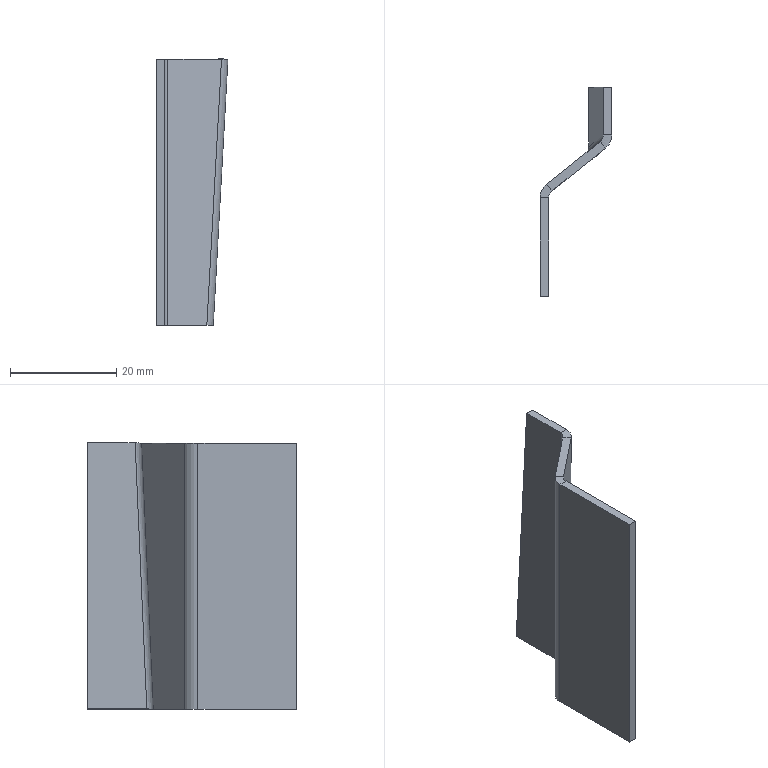Part | SolidWorks | features Fillet 2, Blend 1, FlatPattern 1, SheetMetal 1, SolidToSheetMetal 1 | 1 solid | 22 faces | box 13.5 x 39.3 x 50.088 mm | volume 3525 mm3 | plane 16 | cylinder 4 | spline 2 | commonest cylinder face diameters 3.2 x2 6.4 x2
STEP:
#1=CARTESIAN_POINT('',(-0.3965,21.031,50.));
#2=VERTEX_POINT('',#1);
#3=CARTESIAN_POINT('',(0.6018,19.78,50.));
#4=VERTEX_POINT('',#3);
#5=CARTESIAN_POINT('',(-0.3965,21.031,50.));
#6=CARTESIAN_POINT('',(-0.06372,20.614,50.));
#7=CARTESIAN_POINT('',(0.269,20.197,50.));
#8=CARTESIAN_POINT('',(0.6018,19.78,50.));
#9=B_SPLINE_CURVE_WITH_KNOTS('',3,(#5,#6,#7,#8),.UNSPECIFIED.,.F.,.F.,(4,4),(0.,1.),.UNSPECIFIED.);
#10=EDGE_CURVE('',#2,#4,#9,.T.);
#11=ORIENTED_EDGE('',*,*,#10,.F.);
#12=CARTESIAN_POINT('',(-1.6,18.53,50.));
#13=VERTEX_POINT('',#12);
#14=CARTESIAN_POINT('',(1.6,18.53,50.));
#15=DIRECTION('',(0.,0.,-1.));
#16=DIRECTION('',(0.,-1.,0.));
#17=AXIS2_PLACEMENT_3D('',#14,#15,#16);
#18=CIRCLE('',#17,3.2);
#19=EDGE_CURVE('',#13,#2,#18,.T.);
#20=ORIENTED_EDGE('',*,*,#19,.F.);
#21=CARTESIAN_POINT('',(0.,18.53,50.));
#22=VERTEX_POINT('',#21);
#23=CARTESIAN_POINT('',(-1.6,18.53,50.));
#24=CARTESIAN_POINT('',(-1.067,18.53,50.));
#25=CARTESIAN_POINT('',(-0.5333,18.53,50.));
#26=CARTESIAN_POINT('',(0.,18.53,50.));
#27=B_SPLINE_CURVE_WITH_KNOTS('',3,(#23,#24,#25,#26),.UNSPECIFIED.,.F.,.F.,(4,4),(0.,1.),.UNSPECIFIED.);
#28=EDGE_CURVE('',#13,#22,#27,.T.);
#29=ORIENTED_EDGE('',*,*,#28,.T.);
#30=CARTESIAN_POINT('',(1.6,18.53,50.));
#31=DIRECTION('',(0.,0.,-1.));
#32=DIRECTION('',(-1.,0.,0.));
#33=AXIS2_PLACEMENT_3D('',#30,#31,#32);
#34=CIRCLE('',#33,1.6);
#35=EDGE_CURVE('',#22,#4,#34,.T.);
#36=ORIENTED_EDGE('',*,*,#35,.T.);
#37=EDGE_LOOP('',(#11,#20,#29,#36));
#38=FACE_OUTER_BOUND('',#37,.T.);
#39=CARTESIAN_POINT('',(1.6,18.53,50.));
#40=DIRECTION('',(0.,0.,1.));
#41=DIRECTION('',(1.,0.,0.));
#42=AXIS2_PLACEMENT_3D('',#39,#40,#41);
#43=PLANE('',#42);
#44=ADVANCED_FACE('',(#38),#43,.T.);
#45=ORIENTED_EDGE('',*,*,#28,.F.);
#46=CARTESIAN_POINT('',(-1.6,0.,50.));
#47=VERTEX_POINT('',#46);
#48=CARTESIAN_POINT('',(-1.6,0.,50.));
#49=CARTESIAN_POINT('',(-1.6,6.177,50.));
#50=CARTESIAN_POINT('',(-1.6,12.353,50.));
#51=CARTESIAN_POINT('',(-1.6,18.53,50.));
#52=B_SPLINE_CURVE_WITH_KNOTS('',3,(#48,#49,#50,#51),.UNSPECIFIED.,.F.,.F.,(4,4),(0.03989,1.),.UNSPECIFIED.);
#53=EDGE_CURVE('',#47,#13,#52,.T.);
#54=ORIENTED_EDGE('',*,*,#53,.F.);
#55=CARTESIAN_POINT('',(0.,0.,50.));
#56=VERTEX_POINT('',#55);
#57=CARTESIAN_POINT('',(-1.6,0.,50.));
#58=CARTESIAN_POINT('',(-1.067,0.,50.));
#59=CARTESIAN_POINT('',(-0.5333,0.,50.));
#60=CARTESIAN_POINT('',(0.,0.,50.));
#61=B_SPLINE_CURVE_WITH_KNOTS('',3,(#57,#58,#59,#60),.UNSPECIFIED.,.F.,.F.,(4,4),(0.,1.),.UNSPECIFIED.);
#62=EDGE_CURVE('',#47,#56,#61,.T.);
#63=ORIENTED_EDGE('',*,*,#62,.T.);
#64=CARTESIAN_POINT('',(0.,0.,50.));
#65=DIRECTION('',(0.,1.,0.));
#66=VECTOR('',#65,1000.);
#67=LINE('',#64,#66);
#68=EDGE_CURVE('',#56,#22,#67,.T.);
#69=ORIENTED_EDGE('',*,*,#68,.T.);
#70=EDGE_LOOP('',(#45,#54,#63,#69));
#71=FACE_OUTER_BOUND('',#70,.T.);
#72=CARTESIAN_POINT('',(0.,18.53,50.));
#73=DIRECTION('',(0.,0.,1.));
#74=DIRECTION('',(-1.,0.,0.));
#75=AXIS2_PLACEMENT_3D('',#72,#73,#74);
#76=PLANE('',#75);
#77=ADVANCED_FACE('',(#71),#76,.T.);
#78=ORIENTED_EDGE('',*,*,#62,.F.);
#79=CARTESIAN_POINT('',(-1.6,0.,0.));
#80=VERTEX_POINT('',#79);
#81=CARTESIAN_POINT('',(-1.6,0.,0.));
#82=DIRECTION('',(0.,0.,-1.));
#83=VECTOR('',#82,1000.);
#84=LINE('',#81,#83);
#85=EDGE_CURVE('',#47,#80,#84,.T.);
#86=ORIENTED_EDGE('',*,*,#85,.T.);
#87=CARTESIAN_POINT('',(0.,0.,0.));
#88=VERTEX_POINT('',#87);
#89=CARTESIAN_POINT('',(-1.6,0.,0.));
#90=CARTESIAN_POINT('',(-1.067,0.,0.));
#91=CARTESIAN_POINT('',(-0.5333,0.,0.));
#92=CARTESIAN_POINT('',(0.,0.,0.));
#93=B_SPLINE_CURVE_WITH_KNOTS('',3,(#89,#90,#91,#92),.UNSPECIFIED.,.F.,.F.,(4,4),(0.,1.),.UNSPECIFIED.);
#94=EDGE_CURVE('',#80,#88,#93,.T.);
#95=ORIENTED_EDGE('',*,*,#94,.T.);
#96=CARTESIAN_POINT('',(0.,0.,50.));
#97=DIRECTION('',(0.,0.,-1.));
#98=VECTOR('',#97,1000.);
#99=LINE('',#96,#98);
#100=EDGE_CURVE('',#56,#88,#99,.T.);
#101=ORIENTED_EDGE('',*,*,#100,.F.);
#102=EDGE_LOOP('',(#78,#86,#95,#101));
#103=FACE_OUTER_BOUND('',#102,.T.);
#104=CARTESIAN_POINT('',(0.,0.,50.));
#105=DIRECTION('',(0.,-1.,0.));
#106=DIRECTION('',(0.,0.,-1.));
#107=AXIS2_PLACEMENT_3D('',#104,#105,#106);
#108=PLANE('',#107);
#109=ADVANCED_FACE('',(#103),#108,.T.);
#110=ORIENTED_EDGE('',*,*,#94,.F.);
#111=CARTESIAN_POINT('',(-1.6,18.53,0.));
#112=VERTEX_POINT('',#111);
#113=CARTESIAN_POINT('',(-1.6,0.,0.));
#114=CARTESIAN_POINT('',(-1.6,6.177,0.));
#115=CARTESIAN_POINT('',(-1.6,12.353,0.));
#116=CARTESIAN_POINT('',(-1.6,18.53,0.));
#117=B_SPLINE_CURVE_WITH_KNOTS('',3,(#113,#114,#115,#116),.UNSPECIFIED.,.F.,.F.,(4,4),(0.,1.),.UNSPECIFIED.);
#118=EDGE_CURVE('',#80,#112,#117,.T.);
#119=ORIENTED_EDGE('',*,*,#118,.T.);
#120=CARTESIAN_POINT('',(0.,18.53,0.));
#121=VERTEX_POINT('',#120);
#122=CARTESIAN_POINT('',(-1.6,18.53,0.));
#123=CARTESIAN_POINT('',(-1.067,18.53,0.));
#124=CARTESIAN_POINT('',(-0.5333,18.53,0.));
#125=CARTESIAN_POINT('',(0.,18.53,0.));
#126=B_SPLINE_CURVE_WITH_KNOTS('',3,(#122,#123,#124,#125),.UNSPECIFIED.,.F.,.F.,(4,4),(0.,1.),.UNSPECIFIED.);
#127=EDGE_CURVE('',#112,#121,#126,.T.);
#128=ORIENTED_EDGE('',*,*,#127,.T.);
#129=CARTESIAN_POINT('',(0.,19.3,0.));
#130=DIRECTION('',(0.,1.,0.));
#131=VECTOR('',#130,1000.);
#132=LINE('',#129,#131);
#133=EDGE_CURVE('',#88,#121,#132,.T.);
#134=ORIENTED_EDGE('',*,*,#133,.F.);
#135=EDGE_LOOP('',(#110,#119,#128,#134));
#136=FACE_OUTER_BOUND('',#135,.T.);
#137=CARTESIAN_POINT('',(0.,0.,0.));
#138=DIRECTION('',(0.,0.,-1.));
#139=DIRECTION('',(-1.,0.,0.));
#140=AXIS2_PLACEMENT_3D('',#137,#138,#139);
#141=PLANE('',#140);
#142=ADVANCED_FACE('',(#136),#141,.T.);
#143=ORIENTED_EDGE('',*,*,#127,.F.);
#144=CARTESIAN_POINT('',(-0.3965,21.031,0.));
#145=VERTEX_POINT('',#144);
#146=CARTESIAN_POINT('',(1.6,18.53,0.));
#147=DIRECTION('',(0.,0.,1.));
#148=DIRECTION('',(0.,-1.,0.));
#149=AXIS2_PLACEMENT_3D('',#146,#147,#148);
#150=CIRCLE('',#149,3.2);
#151=EDGE_CURVE('',#145,#112,#150,.T.);
#152=ORIENTED_EDGE('',*,*,#151,.F.);
#153=CARTESIAN_POINT('',(0.6018,19.78,0.));
#154=VERTEX_POINT('',#153);
#155=CARTESIAN_POINT('',(-0.3965,21.031,0.));
#156=CARTESIAN_POINT('',(-0.06372,20.614,0.));
#157=CARTESIAN_POINT('',(0.269,20.197,0.));
#158=CARTESIAN_POINT('',(0.6018,19.78,0.));
#159=B_SPLINE_CURVE_WITH_KNOTS('',3,(#155,#156,#157,#158),.UNSPECIFIED.,.F.,.F.,(4,4),(0.,1.),.UNSPECIFIED.);
#160=EDGE_CURVE('',#145,#154,#159,.T.);
#161=ORIENTED_EDGE('',*,*,#160,.T.);
#162=CARTESIAN_POINT('',(1.6,18.53,0.));
#163=DIRECTION('',(0.,0.,1.));
#164=DIRECTION('',(1.,0.,0.));
#165=AXIS2_PLACEMENT_3D('',#162,#163,#164);
#166=CIRCLE('',#165,1.6);
#167=EDGE_CURVE('',#154,#121,#166,.T.);
#168=ORIENTED_EDGE('',*,*,#167,.T.);
#169=EDGE_LOOP('',(#143,#152,#161,#168));
#170=FACE_OUTER_BOUND('',#169,.T.);
#171=CARTESIAN_POINT('',(1.6,18.53,0.));
#172=DIRECTION('',(0.,0.,-1.));
#173=DIRECTION('',(-1.,0.,0.));
#174=AXIS2_PLACEMENT_3D('',#171,#172,#173);
#175=PLANE('',#174);
#176=ADVANCED_FACE('',(#170),#175,.T.);
#177=ORIENTED_EDGE('',*,*,#160,.F.);
#178=CARTESIAN_POINT('',(6.938,26.886,0.));
#179=VERTEX_POINT('',#178);
#180=CARTESIAN_POINT('',(-0.3965,21.031,0.));
#181=CARTESIAN_POINT('',(2.048,22.982,0.));
#182=CARTESIAN_POINT('',(4.493,24.934,0.));
#183=CARTESIAN_POINT('',(6.938,26.886,0.));
#184=B_SPLINE_CURVE_WITH_KNOTS('',3,(#180,#181,#182,#183),.UNSPECIFIED.,.F.,.F.,(4,4),(0.,1.),.UNSPECIFIED.);
#185=EDGE_CURVE('',#145,#179,#184,.T.);
#186=ORIENTED_EDGE('',*,*,#185,.T.);
#187=CARTESIAN_POINT('',(7.936,25.635,0.));
#188=VERTEX_POINT('',#187);
#189=CARTESIAN_POINT('',(6.938,26.886,0.));
#190=CARTESIAN_POINT('',(7.27,26.469,0.));
#191=CARTESIAN_POINT('',(7.603,26.052,0.));
#192=CARTESIAN_POINT('',(7.936,25.635,0.));
#193=B_SPLINE_CURVE_WITH_KNOTS('',3,(#189,#190,#191,#192),.UNSPECIFIED.,.F.,.F.,(4,4),(0.,1.),.UNSPECIFIED.);
#194=EDGE_CURVE('',#179,#188,#193,.T.);
#195=ORIENTED_EDGE('',*,*,#194,.T.);
#196=CARTESIAN_POINT('',(0.,19.3,0.));
#197=DIRECTION('',(0.7815,0.6239,0.));
#198=VECTOR('',#197,1000.);
#199=LINE('',#196,#198);
#200=EDGE_CURVE('',#154,#188,#199,.T.);
#201=ORIENTED_EDGE('',*,*,#200,.F.);
#202=EDGE_LOOP('',(#177,#186,#195,#201));
#203=FACE_OUTER_BOUND('',#202,.T.);
#204=CARTESIAN_POINT('',(0.6018,19.78,0.));
#205=DIRECTION('',(0.,0.,-1.));
#206=DIRECTION('',(-0.6239,0.7815,0.));
#207=AXIS2_PLACEMENT_3D('',#204,#205,#206);
#208=PLANE('',#207);
#209=ADVANCED_FACE('',(#203),#208,.T.);
#210=ORIENTED_EDGE('',*,*,#194,.F.);
#211=CARTESIAN_POINT('',(7.547,28.144,0.08805));
#212=VERTEX_POINT('',#211);
#213=CARTESIAN_POINT('',(7.547,28.144,0.08805));
#214=CARTESIAN_POINT('',(7.545,27.647,0.06632));
#215=CARTESIAN_POINT('',(7.328,27.197,0.03489));
#216=CARTESIAN_POINT('',(6.938,26.886,0.));
#217=(BOUNDED_CURVE()B_SPLINE_CURVE(3,(#213,#214,#215,#216),.UNSPECIFIED.,.F.,.F.)B_SPLINE_CURVE_WITH_KNOTS((4,4),(3.814,4.712),.UNSPECIFIED.)CURVE()GEOMETRIC_REPRESENTATION_ITEM()RATIONAL_B_SPLINE_CURVE((1.,0.9339,0.9339,1.))REPRESENTATION_ITEM(''));
#218=EDGE_CURVE('',#212,#179,#217,.T.);
#219=ORIENTED_EDGE('',*,*,#218,.F.);
#220=CARTESIAN_POINT('',(9.144,28.144,0.));
#221=VERTEX_POINT('',#220);
#222=CARTESIAN_POINT('',(7.547,28.144,0.08805));
#223=CARTESIAN_POINT('',(8.079,28.144,0.0587));
#224=CARTESIAN_POINT('',(8.612,28.144,0.02935));
#225=CARTESIAN_POINT('',(9.144,28.144,0.));
#226=(BOUNDED_CURVE()B_SPLINE_CURVE(3,(#222,#223,#224,#225),.UNSPECIFIED.,.F.,.F.)B_SPLINE_CURVE_WITH_KNOTS((4,4),(0.,1.),.UNSPECIFIED.)CURVE()GEOMETRIC_REPRESENTATION_ITEM()RATIONAL_B_SPLINE_CURVE((0.6162,0.6162,0.6162,0.6162))REPRESENTATION_ITEM(''));
#227=EDGE_CURVE('',#212,#221,#226,.T.);
#228=ORIENTED_EDGE('',*,*,#227,.T.);
#229=CARTESIAN_POINT('',(9.144,28.144,0.));
#230=CARTESIAN_POINT('',(9.144,27.151,0.));
#231=CARTESIAN_POINT('',(8.713,26.256,0.));
#232=CARTESIAN_POINT('',(7.936,25.635,0.));
#233=(BOUNDED_CURVE()B_SPLINE_CURVE(3,(#229,#230,#231,#232),.UNSPECIFIED.,.F.,.F.)B_SPLINE_CURVE_WITH_KNOTS((4,4),(3.814,4.712),.UNSPECIFIED.)CURVE()GEOMETRIC_REPRESENTATION_ITEM()RATIONAL_B_SPLINE_CURVE((1.,0.9339,0.9339,1.))REPRESENTATION_ITEM(''));
#234=EDGE_CURVE('',#221,#188,#233,.T.);
#235=ORIENTED_EDGE('',*,*,#234,.T.);
#236=EDGE_LOOP('',(#210,#219,#228,#235));
#237=FACE_OUTER_BOUND('',#236,.T.);
#238=CARTESIAN_POINT('',(3.432,26.135,0.));
#239=CARTESIAN_POINT('',(3.848,26.467,-0.03752));
#240=CARTESIAN_POINT('',(4.264,26.799,-0.07504));
#241=CARTESIAN_POINT('',(4.68,27.13,-0.1126));
#242=CARTESIAN_POINT('',(-0.5606,31.136,0.));
#243=CARTESIAN_POINT('',(0.5207,30.635,-0.03752));
#244=CARTESIAN_POINT('',(1.602,30.133,-0.07504));
#245=CARTESIAN_POINT('',(2.683,29.631,-0.1126));
#246=CARTESIAN_POINT('',(4.453,35.139,0.));
#247=CARTESIAN_POINT('',(4.703,33.974,0.03752));
#248=CARTESIAN_POINT('',(4.953,32.808,0.07504));
#249=CARTESIAN_POINT('',(5.203,31.643,0.1126));
#250=CARTESIAN_POINT('',(8.446,30.138,0.));
#251=CARTESIAN_POINT('',(8.031,29.806,0.03752));
#252=CARTESIAN_POINT('',(7.615,29.474,0.07504));
#253=CARTESIAN_POINT('',(7.199,29.142,0.1126));
#254=CARTESIAN_POINT('',(12.439,25.136,0.));
#255=CARTESIAN_POINT('',(11.358,25.638,0.03752));
#256=CARTESIAN_POINT('',(10.277,26.139,0.07504));
#257=CARTESIAN_POINT('',(9.196,26.641,0.1126));
#258=CARTESIAN_POINT('',(7.425,21.133,0.));
#259=CARTESIAN_POINT('',(7.176,22.299,-0.03752));
#260=CARTESIAN_POINT('',(6.926,23.464,-0.07504));
#261=CARTESIAN_POINT('',(6.676,24.63,-0.1126));
#262=CARTESIAN_POINT('',(3.432,26.135,0.));
#263=CARTESIAN_POINT('',(3.848,26.467,-0.03752));
#264=CARTESIAN_POINT('',(4.264,26.799,-0.07504));
#265=CARTESIAN_POINT('',(4.68,27.13,-0.1126));
#266=(BOUNDED_SURFACE()B_SPLINE_SURFACE(3,3,((#238,#239,#240,#241),(#242,#243,#244,#245),(#246,#247,#248,#249),(#250,#251,#252,#253),(#254,#255,#256,#257),(#258,#259,#260,#261),(#262,#263,#264,#265)),.UNSPECIFIED.,.T.,.F.,.F.)B_SPLINE_SURFACE_WITH_KNOTS((4,3,4),(4,4),(0.,0.5,1.),(0.,1.),.UNSPECIFIED.)GEOMETRIC_REPRESENTATION_ITEM()RATIONAL_B_SPLINE_SURFACE(((1.,1.,1.,1.),(0.3333,0.3333,0.3333,0.3333),(0.3333,0.3333,0.3333,0.3333),(1.,1.,1.,1.),(0.3333,0.3333,0.3333,0.3333),(0.3333,0.3333,0.3333,0.3333),(1.,1.,1.,1.)))REPRESENTATION_ITEM('')SURFACE());
#267=ADVANCED_FACE('',(#237),#266,.T.);
#268=ORIENTED_EDGE('',*,*,#227,.F.);
#269=CARTESIAN_POINT('',(7.547,39.3,0.08805));
#270=VERTEX_POINT('',#269);
#271=CARTESIAN_POINT('',(7.547,28.144,0.08805));
#272=CARTESIAN_POINT('',(7.547,31.863,0.08805));
#273=CARTESIAN_POINT('',(7.547,35.581,0.08805));
#274=CARTESIAN_POINT('',(7.547,39.3,0.08805));
#275=B_SPLINE_CURVE_WITH_KNOTS('',3,(#271,#272,#273,#274),.UNSPECIFIED.,.F.,.F.,(4,4),(0.,1.),.UNSPECIFIED.);
#276=EDGE_CURVE('',#212,#270,#275,.T.);
#277=ORIENTED_EDGE('',*,*,#276,.T.);
#278=CARTESIAN_POINT('',(9.144,39.3,0.));
#279=VERTEX_POINT('',#278);
#280=CARTESIAN_POINT('',(7.547,39.3,0.08805));
#281=CARTESIAN_POINT('',(8.079,39.3,0.0587));
#282=CARTESIAN_POINT('',(8.612,39.3,0.02935));
#283=CARTESIAN_POINT('',(9.144,39.3,0.));
#284=B_SPLINE_CURVE_WITH_KNOTS('',3,(#280,#281,#282,#283),.UNSPECIFIED.,.F.,.F.,(4,4),(0.,1.),.UNSPECIFIED.);
#285=EDGE_CURVE('',#270,#279,#284,.T.);
#286=ORIENTED_EDGE('',*,*,#285,.T.);
#287=CARTESIAN_POINT('',(9.144,39.3,0.));
#288=DIRECTION('',(0.,1.,0.));
#289=VECTOR('',#288,1000.);
#290=LINE('',#287,#289);
#291=EDGE_CURVE('',#221,#279,#290,.T.);
#292=ORIENTED_EDGE('',*,*,#291,.F.);
#293=EDGE_LOOP('',(#268,#277,#286,#292));
#294=FACE_OUTER_BOUND('',#293,.T.);
#295=CARTESIAN_POINT('',(9.144,28.144,0.));
#296=DIRECTION('',(-0.05503,0.,-0.9985));
#297=DIRECTION('',(-0.9985,0.,0.05503));
#298=AXIS2_PLACEMENT_3D('',#295,#296,#297);
#299=PLANE('',#298);
#300=ADVANCED_FACE('',(#294),#299,.T.);
#301=ORIENTED_EDGE('',*,*,#285,.F.);
#302=CARTESIAN_POINT('',(10.302,39.3,50.088));
#303=VERTEX_POINT('',#302);
#304=CARTESIAN_POINT('',(7.519,39.3,-0.4144));
#305=DIRECTION('',(-0.05503,0.,-0.9985));
#306=VECTOR('',#305,1000.);
#307=LINE('',#304,#306);
#308=EDGE_CURVE('',#303,#270,#307,.T.);
#309=ORIENTED_EDGE('',*,*,#308,.F.);
#310=CARTESIAN_POINT('',(11.9,39.3,50.));
#311=VERTEX_POINT('',#310);
#312=CARTESIAN_POINT('',(10.302,39.3,50.088));
#313=CARTESIAN_POINT('',(10.835,39.3,50.059));
#314=CARTESIAN_POINT('',(11.367,39.3,50.029));
#315=CARTESIAN_POINT('',(11.9,39.3,50.));
#316=B_SPLINE_CURVE_WITH_KNOTS('',3,(#312,#313,#314,#315),.UNSPECIFIED.,.F.,.F.,(4,4),(0.,1.),.UNSPECIFIED.);
#317=EDGE_CURVE('',#303,#311,#316,.T.);
#318=ORIENTED_EDGE('',*,*,#317,.T.);
#319=CARTESIAN_POINT('',(11.9,39.3,50.));
#320=DIRECTION('',(-0.05503,0.,-0.9985));
#321=VECTOR('',#320,1000.);
#322=LINE('',#319,#321);
#323=EDGE_CURVE('',#311,#279,#322,.T.);
#324=ORIENTED_EDGE('',*,*,#323,.T.);
#325=EDGE_LOOP('',(#301,#309,#318,#324));
#326=FACE_OUTER_BOUND('',#325,.T.);
#327=CARTESIAN_POINT('',(11.9,39.3,50.));
#328=DIRECTION('',(0.,-1.,0.));
#329=DIRECTION('',(-0.05503,0.,-0.9985));
#330=AXIS2_PLACEMENT_3D('',#327,#328,#329);
#331=PLANE('',#330);
#332=ADVANCED_FACE('',(#326),#331,.F.);
#333=ORIENTED_EDGE('',*,*,#317,.F.);
#334=CARTESIAN_POINT('',(10.302,30.344,50.088));
#335=VERTEX_POINT('',#334);
#336=CARTESIAN_POINT('',(10.302,30.344,50.088));
#337=CARTESIAN_POINT('',(10.302,33.329,50.088));
#338=CARTESIAN_POINT('',(10.302,36.315,50.088));
#339=CARTESIAN_POINT('',(10.302,39.3,50.088));
#340=B_SPLINE_CURVE_WITH_KNOTS('',3,(#336,#337,#338,#339),.UNSPECIFIED.,.F.,.F.,(4,4),(0.0000024,0.853),.UNSPECIFIED.);
#341=EDGE_CURVE('',#335,#303,#340,.T.);
#342=ORIENTED_EDGE('',*,*,#341,.F.);
#343=CARTESIAN_POINT('',(11.9,30.344,50.));
#344=VERTEX_POINT('',#343);
#345=CARTESIAN_POINT('',(10.302,30.344,50.088));
#346=CARTESIAN_POINT('',(10.835,30.344,50.059));
#347=CARTESIAN_POINT('',(11.367,30.344,50.029));
#348=CARTESIAN_POINT('',(11.9,30.344,50.));
#349=B_SPLINE_CURVE_WITH_KNOTS('',3,(#345,#346,#347,#348),.UNSPECIFIED.,.F.,.F.,(4,4),(0.,1.),.UNSPECIFIED.);
#350=EDGE_CURVE('',#335,#344,#349,.T.);
#351=ORIENTED_EDGE('',*,*,#350,.T.);
#352=CARTESIAN_POINT('',(11.9,39.3,50.));
#353=DIRECTION('',(0.,1.,0.));
#354=VECTOR('',#353,1000.);
#355=LINE('',#352,#354);
#356=EDGE_CURVE('',#344,#311,#355,.T.);
#357=ORIENTED_EDGE('',*,*,#356,.T.);
#358=EDGE_LOOP('',(#333,#342,#351,#357));
#359=FACE_OUTER_BOUND('',#358,.T.);
#360=CARTESIAN_POINT('',(11.9,39.3,50.));
#361=DIRECTION('',(0.05503,0.,0.9985));
#362=DIRECTION('',(-0.9985,0.,0.05503));
#363=AXIS2_PLACEMENT_3D('',#360,#361,#362);
#364=PLANE('',#363);
#365=ADVANCED_FACE('',(#359),#364,.T.);
#366=ORIENTED_EDGE('',*,*,#350,.F.);
#367=CARTESIAN_POINT('',(9.693,29.086,50.));
#368=VERTEX_POINT('',#367);
#369=CARTESIAN_POINT('',(9.693,29.086,50.));
#370=CARTESIAN_POINT('',(10.084,29.397,50.035));
#371=CARTESIAN_POINT('',(10.301,29.847,50.066));
#372=CARTESIAN_POINT('',(10.302,30.344,50.088));
#373=(BOUNDED_CURVE()B_SPLINE_CURVE(3,(#369,#370,#371,#372),.UNSPECIFIED.,.F.,.F.)B_SPLINE_CURVE_WITH_KNOTS((4,4),(1.571,2.469),.UNSPECIFIED.)CURVE()GEOMETRIC_REPRESENTATION_ITEM()RATIONAL_B_SPLINE_CURVE((1.,0.9339,0.9339,1.))REPRESENTATION_ITEM(''));
#374=EDGE_CURVE('',#368,#335,#373,.T.);
#375=ORIENTED_EDGE('',*,*,#374,.F.);
#376=CARTESIAN_POINT('',(10.692,27.835,50.));
#377=VERTEX_POINT('',#376);
#378=CARTESIAN_POINT('',(9.693,29.086,50.));
#379=CARTESIAN_POINT('',(10.026,28.669,50.));
#380=CARTESIAN_POINT('',(10.359,28.252,50.));
#381=CARTESIAN_POINT('',(10.692,27.835,50.));
#382=(BOUNDED_CURVE()B_SPLINE_CURVE(3,(#378,#379,#380,#381),.UNSPECIFIED.,.F.,.F.)B_SPLINE_CURVE_WITH_KNOTS((4,4),(0.,1.),.UNSPECIFIED.)CURVE()GEOMETRIC_REPRESENTATION_ITEM()RATIONAL_B_SPLINE_CURVE((0.5,0.5,0.5,0.5))REPRESENTATION_ITEM(''));
#383=EDGE_CURVE('',#368,#377,#382,.T.);
#384=ORIENTED_EDGE('',*,*,#383,.T.);
#385=CARTESIAN_POINT('',(10.692,27.835,50.));
#386=CARTESIAN_POINT('',(11.469,28.456,50.));
#387=CARTESIAN_POINT('',(11.9,29.351,50.));
#388=CARTESIAN_POINT('',(11.9,30.344,50.));
#389=(BOUNDED_CURVE()B_SPLINE_CURVE(3,(#385,#386,#387,#388),.UNSPECIFIED.,.F.,.F.)B_SPLINE_CURVE_WITH_KNOTS((4,4),(1.571,2.469),.UNSPECIFIED.)CURVE()GEOMETRIC_REPRESENTATION_ITEM()RATIONAL_B_SPLINE_CURVE((1.,0.9339,0.9339,1.))REPRESENTATION_ITEM(''));
#390=EDGE_CURVE('',#377,#344,#389,.T.);
#391=ORIENTED_EDGE('',*,*,#390,.T.);
#392=EDGE_LOOP('',(#366,#375,#384,#391));
#393=FACE_OUTER_BOUND('',#392,.T.);
#394=CARTESIAN_POINT('',(6.188,28.335,50.));
#395=CARTESIAN_POINT('',(6.604,28.667,49.962));
#396=CARTESIAN_POINT('',(7.02,28.999,49.925));
#397=CARTESIAN_POINT('',(7.435,29.33,49.887));
#398=CARTESIAN_POINT('',(10.181,23.333,50.));
#399=CARTESIAN_POINT('',(9.931,24.499,49.962));
#400=CARTESIAN_POINT('',(9.682,25.664,49.925));
#401=CARTESIAN_POINT('',(9.432,26.83,49.887));
#402=CARTESIAN_POINT('',(15.195,27.336,50.));
#403=CARTESIAN_POINT('',(14.114,27.838,50.038));
#404=CARTESIAN_POINT('',(13.033,28.339,50.075));
#405=CARTESIAN_POINT('',(11.951,28.841,50.113));
#406=CARTESIAN_POINT('',(11.202,32.338,50.));
#407=CARTESIAN_POINT('',(10.786,32.006,50.038));
#408=CARTESIAN_POINT('',(10.371,31.674,50.075));
#409=CARTESIAN_POINT('',(9.955,31.342,50.113));
#410=CARTESIAN_POINT('',(7.209,37.339,50.));
#411=CARTESIAN_POINT('',(7.459,36.174,50.038));
#412=CARTESIAN_POINT('',(7.709,35.008,50.075));
#413=CARTESIAN_POINT('',(7.958,33.843,50.113));
#414=CARTESIAN_POINT('',(2.195,33.336,50.));
#415=CARTESIAN_POINT('',(3.276,32.835,49.962));
#416=CARTESIAN_POINT('',(4.358,32.333,49.925));
#417=CARTESIAN_POINT('',(5.439,31.831,49.887));
#418=CARTESIAN_POINT('',(6.188,28.335,50.));
#419=CARTESIAN_POINT('',(6.604,28.667,49.962));
#420=CARTESIAN_POINT('',(7.02,28.999,49.925));
#421=CARTESIAN_POINT('',(7.435,29.33,49.887));
#422=(BOUNDED_SURFACE()B_SPLINE_SURFACE(3,3,((#394,#395,#396,#397),(#398,#399,#400,#401),(#402,#403,#404,#405),(#406,#407,#408,#409),(#410,#411,#412,#413),(#414,#415,#416,#417),(#418,#419,#420,#421)),.UNSPECIFIED.,.T.,.F.,.F.)B_SPLINE_SURFACE_WITH_KNOTS((4,3,4),(4,4),(0.,0.5,1.),(0.,1.),.UNSPECIFIED.)GEOMETRIC_REPRESENTATION_ITEM()RATIONAL_B_SPLINE_SURFACE(((1.,1.,1.,1.),(0.3333,0.3333,0.3333,0.3333),(0.3333,0.3333,0.3333,0.3333),(1.,1.,1.,1.),(0.3333,0.3333,0.3333,0.3333),(0.3333,0.3333,0.3333,0.3333),(1.,1.,1.,1.)))REPRESENTATION_ITEM('')SURFACE());
#423=ADVANCED_FACE('',(#393),#422,.T.);
#424=CARTESIAN_POINT('',(-0.3965,21.031,50.));
#425=CARTESIAN_POINT('',(2.967,23.716,50.));
#426=CARTESIAN_POINT('',(6.33,26.401,50.));
#427=CARTESIAN_POINT('',(9.693,29.086,50.));
#428=B_SPLINE_CURVE_WITH_KNOTS('',3,(#424,#425,#426,#427),.UNSPECIFIED.,.F.,.F.,(4,4),(0.1015,0.9494),.UNSPECIFIED.);
#429=EDGE_CURVE('',#2,#368,#428,.T.);
#430=ORIENTED_EDGE('',*,*,#429,.F.);
#431=ORIENTED_EDGE('',*,*,#10,.T.);
#432=CARTESIAN_POINT('',(0.,19.3,50.));
#433=DIRECTION('',(0.7815,0.6239,0.));
#434=VECTOR('',#433,1000.);
#435=LINE('',#432,#434);
#436=EDGE_CURVE('',#4,#377,#435,.T.);
#437=ORIENTED_EDGE('',*,*,#436,.T.);
#438=ORIENTED_EDGE('',*,*,#383,.F.);
#439=EDGE_LOOP('',(#430,#431,#437,#438));
#440=FACE_OUTER_BOUND('',#439,.T.);
#441=CARTESIAN_POINT('',(10.692,27.835,50.));
#442=DIRECTION('',(0.,0.,1.));
#443=DIRECTION('',(-0.6239,0.7815,0.));
#444=AXIS2_PLACEMENT_3D('',#441,#442,#443);
#445=PLANE('',#444);
#446=ADVANCED_FACE('',(#440),#445,.T.);
#447=ORIENTED_EDGE('',*,*,#390,.F.);
#448=CARTESIAN_POINT('',(7.85,25.567,-1.558));
#449=DIRECTION('',(0.05498,0.04389,0.9975));
#450=VECTOR('',#449,1000.);
#451=LINE('',#448,#450);
#452=EDGE_CURVE('',#188,#377,#451,.T.);
#453=ORIENTED_EDGE('',*,*,#452,.F.);
#454=ORIENTED_EDGE('',*,*,#234,.F.);
#455=CARTESIAN_POINT('',(9.049,28.068,-1.734));
#456=DIRECTION('',(-0.05498,-0.04389,-0.9975));
#457=VECTOR('',#456,1000.);
#458=LINE('',#455,#457);
#459=EDGE_CURVE('',#344,#221,#458,.T.);
#460=ORIENTED_EDGE('',*,*,#459,.F.);
#461=EDGE_LOOP('',(#447,#453,#454,#460));
#462=FACE_OUTER_BOUND('',#461,.T.);
#463=CARTESIAN_POINT('',(5.854,28.068,-1.558));
#464=DIRECTION('',(-0.05498,-0.04389,-0.9975));
#465=DIRECTION('',(-0.9985,0.,0.05503));
#466=AXIS2_PLACEMENT_3D('',#463,#464,#465);
#467=CYLINDRICAL_SURFACE('',#466,3.2);
#468=ADVANCED_FACE('',(#462),#467,.T.);
#469=ORIENTED_EDGE('',*,*,#356,.F.);
#470=ORIENTED_EDGE('',*,*,#459,.T.);
#471=ORIENTED_EDGE('',*,*,#291,.T.);
#472=ORIENTED_EDGE('',*,*,#323,.F.);
#473=EDGE_LOOP('',(#469,#470,#471,#472));
#474=FACE_OUTER_BOUND('',#473,.T.);
#475=CARTESIAN_POINT('',(9.117,0.,-0.5025));
#476=DIRECTION('',(0.9985,0.,-0.05503));
#477=DIRECTION('',(-0.05503,0.,-0.9985));
#478=AXIS2_PLACEMENT_3D('',#475,#476,#477);
#479=PLANE('',#478);
#480=ADVANCED_FACE('',(#474),#479,.T.);
#481=ORIENTED_EDGE('',*,*,#35,.F.);
#482=CARTESIAN_POINT('',(0.,18.53,50.));
#483=DIRECTION('',(0.,0.,1.));
#484=VECTOR('',#483,1000.);
#485=LINE('',#482,#484);
#486=EDGE_CURVE('',#121,#22,#485,.T.);
#487=ORIENTED_EDGE('',*,*,#486,.F.);
#488=ORIENTED_EDGE('',*,*,#167,.F.);
#489=CARTESIAN_POINT('',(0.6018,19.78,0.));
#490=DIRECTION('',(0.,0.,-1.));
#491=VECTOR('',#490,1000.);
#492=LINE('',#489,#491);
#493=EDGE_CURVE('',#4,#154,#492,.T.);
#494=ORIENTED_EDGE('',*,*,#493,.F.);
#495=EDGE_LOOP('',(#481,#487,#488,#494));
#496=FACE_OUTER_BOUND('',#495,.T.);
#497=CARTESIAN_POINT('',(1.6,18.53,0.));
#498=DIRECTION('',(0.,0.,1.));
#499=DIRECTION('',(0.,-1.,0.));
#500=AXIS2_PLACEMENT_3D('',#497,#498,#499);
#501=CYLINDRICAL_SURFACE('',#500,1.6);
#502=ADVANCED_FACE('',(#496),#501,.F.);
#503=ORIENTED_EDGE('',*,*,#200,.T.);
#504=ORIENTED_EDGE('',*,*,#452,.T.);
#505=ORIENTED_EDGE('',*,*,#436,.F.);
#506=ORIENTED_EDGE('',*,*,#493,.T.);
#507=EDGE_LOOP('',(#503,#504,#505,#506));
#508=FACE_OUTER_BOUND('',#507,.T.);
#509=CARTESIAN_POINT('',(-9.41,11.788,0.));
#510=DIRECTION('',(0.6239,-0.7815,0.));
#511=DIRECTION('',(0.7815,0.6239,0.));
#512=AXIS2_PLACEMENT_3D('',#509,#510,#511);
#513=PLANE('',#512);
#514=ADVANCED_FACE('',(#508),#513,.T.);
#515=ORIENTED_EDGE('',*,*,#133,.T.);
#516=ORIENTED_EDGE('',*,*,#486,.T.);
#517=ORIENTED_EDGE('',*,*,#68,.F.);
#518=ORIENTED_EDGE('',*,*,#100,.T.);
#519=EDGE_LOOP('',(#515,#516,#517,#518));
#520=FACE_OUTER_BOUND('',#519,.T.);
#521=CARTESIAN_POINT('',(0.,0.,0.));
#522=DIRECTION('',(1.,0.,0.));
#523=DIRECTION('',(0.,1.,0.));
#524=AXIS2_PLACEMENT_3D('',#521,#522,#523);
#525=PLANE('',#524);
#526=ADVANCED_FACE('',(#520),#525,.T.);
#527=ORIENTED_EDGE('',*,*,#374,.T.);
#528=CARTESIAN_POINT('',(7.451,28.068,-1.646));
#529=DIRECTION('',(-0.05498,-0.04389,-0.9975));
#530=VECTOR('',#529,1000.);
#531=LINE('',#528,#530);
#532=EDGE_CURVE('',#335,#212,#531,.T.);
#533=ORIENTED_EDGE('',*,*,#532,.T.);
#534=ORIENTED_EDGE('',*,*,#218,.T.);
#535=CARTESIAN_POINT('',(6.852,26.817,-1.558));
#536=DIRECTION('',(0.05498,0.04389,0.9975));
#537=VECTOR('',#536,1000.);
#538=LINE('',#535,#537);
#539=EDGE_CURVE('',#179,#368,#538,.T.);
#540=ORIENTED_EDGE('',*,*,#539,.T.);
#541=EDGE_LOOP('',(#527,#533,#534,#540));
#542=FACE_OUTER_BOUND('',#541,.T.);
#543=CARTESIAN_POINT('',(5.854,28.068,-1.558));
#544=DIRECTION('',(-0.05498,-0.04389,-0.9975));
#545=DIRECTION('',(-0.9985,0.,0.05503));
#546=AXIS2_PLACEMENT_3D('',#543,#544,#545);
#547=CYLINDRICAL_SURFACE('',#546,1.6);
#548=ADVANCED_FACE('',(#542),#547,.F.);
#549=ORIENTED_EDGE('',*,*,#341,.T.);
#550=ORIENTED_EDGE('',*,*,#308,.T.);
#551=ORIENTED_EDGE('',*,*,#276,.F.);
#552=ORIENTED_EDGE('',*,*,#532,.F.);
#553=EDGE_LOOP('',(#549,#550,#551,#552));
#554=FACE_OUTER_BOUND('',#553,.T.);
#555=CARTESIAN_POINT('',(7.519,0.,-0.4144));
#556=DIRECTION('',(0.9985,0.,-0.05503));
#557=DIRECTION('',(-0.05503,0.,-0.9985));
#558=AXIS2_PLACEMENT_3D('',#555,#556,#557);
#559=PLANE('',#558);
#560=ADVANCED_FACE('',(#554),#559,.F.);
#561=ORIENTED_EDGE('',*,*,#19,.T.);
#562=CARTESIAN_POINT('',(-0.3965,21.031,0.));
#563=DIRECTION('',(0.,0.,-1.));
#564=VECTOR('',#563,1000.);
#565=LINE('',#562,#564);
#566=EDGE_CURVE('',#2,#145,#565,.T.);
#567=ORIENTED_EDGE('',*,*,#566,.T.);
#568=ORIENTED_EDGE('',*,*,#151,.T.);
#569=CARTESIAN_POINT('',(-1.6,18.53,0.));
#570=DIRECTION('',(0.,0.,1.));
#571=VECTOR('',#570,1000.);
#572=LINE('',#569,#571);
#573=EDGE_CURVE('',#112,#13,#572,.T.);
#574=ORIENTED_EDGE('',*,*,#573,.T.);
#575=EDGE_LOOP('',(#561,#567,#568,#574));
#576=FACE_OUTER_BOUND('',#575,.T.);
#577=CARTESIAN_POINT('',(1.6,18.53,0.));
#578=DIRECTION('',(0.,0.,1.));
#579=DIRECTION('',(0.,-1.,0.));
#580=AXIS2_PLACEMENT_3D('',#577,#578,#579);
#581=CYLINDRICAL_SURFACE('',#580,3.2);
#582=ADVANCED_FACE('',(#576),#581,.T.);
#583=ORIENTED_EDGE('',*,*,#185,.F.);
#584=ORIENTED_EDGE('',*,*,#566,.F.);
#585=ORIENTED_EDGE('',*,*,#429,.T.);
#586=ORIENTED_EDGE('',*,*,#539,.F.);
#587=EDGE_LOOP('',(#583,#584,#585,#586));
#588=FACE_OUTER_BOUND('',#587,.T.);
#589=CARTESIAN_POINT('',(-10.408,13.038,0.));
#590=DIRECTION('',(0.6239,-0.7815,0.));
#591=DIRECTION('',(0.7815,0.6239,0.));
#592=AXIS2_PLACEMENT_3D('',#589,#590,#591);
#593=PLANE('',#592);
#594=ADVANCED_FACE('',(#588),#593,.F.);
#595=ORIENTED_EDGE('',*,*,#118,.F.);
#596=ORIENTED_EDGE('',*,*,#85,.F.);
#597=ORIENTED_EDGE('',*,*,#53,.T.);
#598=ORIENTED_EDGE('',*,*,#573,.F.);
#599=EDGE_LOOP('',(#595,#596,#597,#598));
#600=FACE_OUTER_BOUND('',#599,.T.);
#601=CARTESIAN_POINT('',(-1.6,0.,0.));
#602=DIRECTION('',(1.,0.,0.));
#603=DIRECTION('',(0.,1.,0.));
#604=AXIS2_PLACEMENT_3D('',#601,#602,#603);
#605=PLANE('',#604);
#606=ADVANCED_FACE('',(#600),#605,.F.);
#607=CLOSED_SHELL('',(#44,#77,#109,#142,#176,#209,#267,#300,#332,#365,#423,#446,#468,#480,#502,#514,#526,#548,#560,#582,#594,#606));
#608=MANIFOLD_SOLID_BREP('',#607);
#609=CARTESIAN_POINT('',(0.,0.,0.));
#610=DIRECTION('',(0.,0.,1.));
#611=DIRECTION('',(1.,0.,0.));
#612=AXIS2_PLACEMENT_3D('',#609,#610,#611);
#613=(LENGTH_UNIT()NAMED_UNIT(*)SI_UNIT(.MILLI.,.METRE.));
#614=UNCERTAINTY_MEASURE_WITH_UNIT(LENGTH_MEASURE(0.00001),#613,'','');
#615=(NAMED_UNIT(*)PLANE_ANGLE_UNIT()SI_UNIT($,.RADIAN.));
#616=(NAMED_UNIT(*)SI_UNIT($,.STERADIAN.)SOLID_ANGLE_UNIT());
#617=(GEOMETRIC_REPRESENTATION_CONTEXT(3)GLOBAL_UNCERTAINTY_ASSIGNED_CONTEXT((#614))GLOBAL_UNIT_ASSIGNED_CONTEXT((#613,#615,#616))REPRESENTATION_CONTEXT('',''));
#618=ADVANCED_BREP_SHAPE_REPRESENTATION('',(#608,#612),#617);